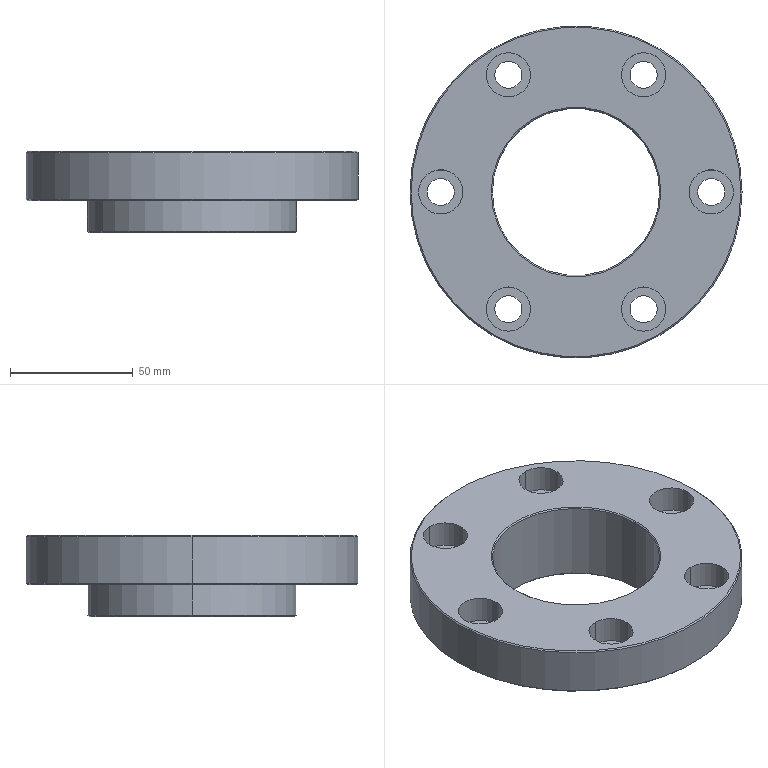Part | SolidWorks | features Chamfer 1, CirPattern 1, HoleWzd 1, Revolution 1 | 1 solid | 49 faces | box 135 x 135 x 33 mm | volume 218081 mm3 | cylinder 30 | cone 10 | plane 9 | commonest cylinder face diameters 11 x12 18 x12 68 x2 85 x2 135 x2
STEP:
#1=CARTESIAN_POINT('',(67.,0.,0.));
#2=VERTEX_POINT('',#1);
#3=CARTESIAN_POINT('',(-67.,0.,0.));
#4=VERTEX_POINT('',#3);
#5=CARTESIAN_POINT('',(0.,0.,0.));
#6=DIRECTION('',(0.,0.,1.));
#7=DIRECTION('',(1.,0.,0.));
#8=AXIS2_PLACEMENT_3D('',#5,#6,#7);
#9=CIRCLE('',#8,67.);
#10=EDGE_CURVE('',#2,#4,#9,.T.);
#11=ORIENTED_EDGE('',*,*,#10,.F.);
#12=CARTESIAN_POINT('',(67.5,0.,-0.5));
#13=VERTEX_POINT('',#12);
#14=CARTESIAN_POINT('',(67.5,0.,-0.5));
#15=DIRECTION('',(0.7071,0.,-0.7071));
#16=VECTOR('',#15,1000.);
#17=LINE('',#14,#16);
#18=EDGE_CURVE('',#2,#13,#17,.T.);
#19=ORIENTED_EDGE('',*,*,#18,.T.);
#20=CARTESIAN_POINT('',(-67.5,0.,-0.5));
#21=VERTEX_POINT('',#20);
#22=CARTESIAN_POINT('',(0.,0.,-0.5));
#23=DIRECTION('',(0.,0.,-1.));
#24=DIRECTION('',(1.,0.,0.));
#25=AXIS2_PLACEMENT_3D('',#22,#23,#24);
#26=CIRCLE('',#25,67.5);
#27=EDGE_CURVE('',#21,#13,#26,.T.);
#28=ORIENTED_EDGE('',*,*,#27,.F.);
#29=CARTESIAN_POINT('',(-67.5,0.,-0.5));
#30=DIRECTION('',(-0.7071,0.,-0.7071));
#31=VECTOR('',#30,1000.);
#32=LINE('',#29,#31);
#33=EDGE_CURVE('',#4,#21,#32,.T.);
#34=ORIENTED_EDGE('',*,*,#33,.F.);
#35=EDGE_LOOP('',(#11,#19,#28,#34));
#36=FACE_OUTER_BOUND('',#35,.T.);
#37=CARTESIAN_POINT('',(0.,0.,-0.5));
#38=DIRECTION('',(0.,0.,-1.));
#39=DIRECTION('',(-1.,0.,0.));
#40=AXIS2_PLACEMENT_3D('',#37,#38,#39);
#41=CONICAL_SURFACE('',#40,67.5,0.7854);
#42=ADVANCED_FACE('',(#36),#41,.T.);
#43=CARTESIAN_POINT('',(-34.,0.,-0.5));
#44=VERTEX_POINT('',#43);
#45=CARTESIAN_POINT('',(34.,0.,-0.5));
#46=VERTEX_POINT('',#45);
#47=CARTESIAN_POINT('',(0.,0.,-0.5));
#48=DIRECTION('',(0.,0.,1.));
#49=DIRECTION('',(1.,0.,0.));
#50=AXIS2_PLACEMENT_3D('',#47,#48,#49);
#51=CIRCLE('',#50,34.);
#52=EDGE_CURVE('',#44,#46,#51,.T.);
#53=ORIENTED_EDGE('',*,*,#52,.F.);
#54=CARTESIAN_POINT('',(-34.5,0.,0.));
#55=VERTEX_POINT('',#54);
#56=CARTESIAN_POINT('',(-34.5,0.,0.));
#57=DIRECTION('',(-0.7071,0.,0.7071));
#58=VECTOR('',#57,1000.);
#59=LINE('',#56,#58);
#60=EDGE_CURVE('',#44,#55,#59,.T.);
#61=ORIENTED_EDGE('',*,*,#60,.T.);
#62=CARTESIAN_POINT('',(34.5,0.,0.));
#63=VERTEX_POINT('',#62);
#64=CARTESIAN_POINT('',(0.,0.,0.));
#65=DIRECTION('',(0.,0.,-1.));
#66=DIRECTION('',(1.,0.,0.));
#67=AXIS2_PLACEMENT_3D('',#64,#65,#66);
#68=CIRCLE('',#67,34.5);
#69=EDGE_CURVE('',#63,#55,#68,.T.);
#70=ORIENTED_EDGE('',*,*,#69,.F.);
#71=CARTESIAN_POINT('',(34.5,0.,0.));
#72=DIRECTION('',(0.7071,0.,0.7071));
#73=VECTOR('',#72,1000.);
#74=LINE('',#71,#73);
#75=EDGE_CURVE('',#46,#63,#74,.T.);
#76=ORIENTED_EDGE('',*,*,#75,.F.);
#77=EDGE_LOOP('',(#53,#61,#70,#76));
#78=FACE_OUTER_BOUND('',#77,.T.);
#79=CARTESIAN_POINT('',(0.,0.,0.));
#80=DIRECTION('',(0.,0.,1.));
#81=DIRECTION('',(1.,0.,0.));
#82=AXIS2_PLACEMENT_3D('',#79,#80,#81);
#83=CONICAL_SURFACE('',#82,34.5,0.7854);
#84=ADVANCED_FACE('',(#78),#83,.F.);
#85=CARTESIAN_POINT('',(-67.,0.,-20.));
#86=VERTEX_POINT('',#85);
#87=CARTESIAN_POINT('',(67.,0.,-20.));
#88=VERTEX_POINT('',#87);
#89=CARTESIAN_POINT('',(0.,0.,-20.));
#90=DIRECTION('',(0.,0.,-1.));
#91=DIRECTION('',(-1.,0.,0.));
#92=AXIS2_PLACEMENT_3D('',#89,#90,#91);
#93=CIRCLE('',#92,67.);
#94=EDGE_CURVE('',#86,#88,#93,.T.);
#95=ORIENTED_EDGE('',*,*,#94,.F.);
#96=CARTESIAN_POINT('',(-67.5,0.,-19.5));
#97=VERTEX_POINT('',#96);
#98=CARTESIAN_POINT('',(-67.,0.,-20.));
#99=DIRECTION('',(-0.7071,0.,0.7071));
#100=VECTOR('',#99,1000.);
#101=LINE('',#98,#100);
#102=EDGE_CURVE('',#86,#97,#101,.T.);
#103=ORIENTED_EDGE('',*,*,#102,.T.);
#104=CARTESIAN_POINT('',(67.5,0.,-19.5));
#105=VERTEX_POINT('',#104);
#106=CARTESIAN_POINT('',(0.,0.,-19.5));
#107=DIRECTION('',(0.,0.,1.));
#108=DIRECTION('',(-1.,0.,0.));
#109=AXIS2_PLACEMENT_3D('',#106,#107,#108);
#110=CIRCLE('',#109,67.5);
#111=EDGE_CURVE('',#105,#97,#110,.T.);
#112=ORIENTED_EDGE('',*,*,#111,.F.);
#113=CARTESIAN_POINT('',(67.,0.,-20.));
#114=DIRECTION('',(0.7071,0.,0.7071));
#115=VECTOR('',#114,1000.);
#116=LINE('',#113,#115);
#117=EDGE_CURVE('',#88,#105,#116,.T.);
#118=ORIENTED_EDGE('',*,*,#117,.F.);
#119=EDGE_LOOP('',(#95,#103,#112,#118));
#120=FACE_OUTER_BOUND('',#119,.T.);
#121=CARTESIAN_POINT('',(0.,0.,-20.));
#122=DIRECTION('',(0.,0.,1.));
#123=DIRECTION('',(1.,0.,0.));
#124=AXIS2_PLACEMENT_3D('',#121,#122,#123);
#125=CONICAL_SURFACE('',#124,67.,0.7854);
#126=ADVANCED_FACE('',(#120),#125,.T.);
#127=CARTESIAN_POINT('',(-42.,0.,-33.));
#128=VERTEX_POINT('',#127);
#129=CARTESIAN_POINT('',(42.,0.,-33.));
#130=VERTEX_POINT('',#129);
#131=CARTESIAN_POINT('',(0.,0.,-33.));
#132=DIRECTION('',(0.,0.,-1.));
#133=DIRECTION('',(-1.,0.,0.));
#134=AXIS2_PLACEMENT_3D('',#131,#132,#133);
#135=CIRCLE('',#134,42.);
#136=EDGE_CURVE('',#128,#130,#135,.T.);
#137=ORIENTED_EDGE('',*,*,#136,.F.);
#138=CARTESIAN_POINT('',(-42.5,0.,-32.5));
#139=VERTEX_POINT('',#138);
#140=CARTESIAN_POINT('',(-42.,0.,-33.));
#141=DIRECTION('',(-0.7071,0.,0.7071));
#142=VECTOR('',#141,1000.);
#143=LINE('',#140,#142);
#144=EDGE_CURVE('',#128,#139,#143,.T.);
#145=ORIENTED_EDGE('',*,*,#144,.T.);
#146=CARTESIAN_POINT('',(42.5,0.,-32.5));
#147=VERTEX_POINT('',#146);
#148=CARTESIAN_POINT('',(0.,0.,-32.5));
#149=DIRECTION('',(0.,0.,1.));
#150=DIRECTION('',(-1.,0.,0.));
#151=AXIS2_PLACEMENT_3D('',#148,#149,#150);
#152=CIRCLE('',#151,42.5);
#153=EDGE_CURVE('',#147,#139,#152,.T.);
#154=ORIENTED_EDGE('',*,*,#153,.F.);
#155=CARTESIAN_POINT('',(42.,0.,-33.));
#156=DIRECTION('',(0.7071,0.,0.7071));
#157=VECTOR('',#156,1000.);
#158=LINE('',#155,#157);
#159=EDGE_CURVE('',#130,#147,#158,.T.);
#160=ORIENTED_EDGE('',*,*,#159,.F.);
#161=EDGE_LOOP('',(#137,#145,#154,#160));
#162=FACE_OUTER_BOUND('',#161,.T.);
#163=CARTESIAN_POINT('',(0.,0.,-33.));
#164=DIRECTION('',(0.,0.,1.));
#165=DIRECTION('',(1.,0.,0.));
#166=AXIS2_PLACEMENT_3D('',#163,#164,#165);
#167=CONICAL_SURFACE('',#166,42.,0.7854);
#168=ADVANCED_FACE('',(#162),#167,.T.);
#169=CARTESIAN_POINT('',(34.,0.,-32.5));
#170=VERTEX_POINT('',#169);
#171=CARTESIAN_POINT('',(-34.,0.,-32.5));
#172=VERTEX_POINT('',#171);
#173=CARTESIAN_POINT('',(0.,0.,-32.5));
#174=DIRECTION('',(0.,0.,-1.));
#175=DIRECTION('',(-1.,0.,0.));
#176=AXIS2_PLACEMENT_3D('',#173,#174,#175);
#177=CIRCLE('',#176,34.);
#178=EDGE_CURVE('',#170,#172,#177,.T.);
#179=ORIENTED_EDGE('',*,*,#178,.F.);
#180=CARTESIAN_POINT('',(34.5,0.,-33.));
#181=VERTEX_POINT('',#180);
#182=CARTESIAN_POINT('',(34.,0.,-32.5));
#183=DIRECTION('',(0.7071,0.,-0.7071));
#184=VECTOR('',#183,1000.);
#185=LINE('',#182,#184);
#186=EDGE_CURVE('',#170,#181,#185,.T.);
#187=ORIENTED_EDGE('',*,*,#186,.T.);
#188=CARTESIAN_POINT('',(-34.5,0.,-33.));
#189=VERTEX_POINT('',#188);
#190=CARTESIAN_POINT('',(0.,0.,-33.));
#191=DIRECTION('',(0.,0.,1.));
#192=DIRECTION('',(-1.,0.,0.));
#193=AXIS2_PLACEMENT_3D('',#190,#191,#192);
#194=CIRCLE('',#193,34.5);
#195=EDGE_CURVE('',#189,#181,#194,.T.);
#196=ORIENTED_EDGE('',*,*,#195,.F.);
#197=CARTESIAN_POINT('',(-34.,0.,-32.5));
#198=DIRECTION('',(-0.7071,0.,-0.7071));
#199=VECTOR('',#198,1000.);
#200=LINE('',#197,#199);
#201=EDGE_CURVE('',#172,#189,#200,.T.);
#202=ORIENTED_EDGE('',*,*,#201,.F.);
#203=EDGE_LOOP('',(#179,#187,#196,#202));
#204=FACE_OUTER_BOUND('',#203,.T.);
#205=CARTESIAN_POINT('',(0.,0.,-32.5));
#206=DIRECTION('',(0.,0.,-1.));
#207=DIRECTION('',(-1.,0.,0.));
#208=AXIS2_PLACEMENT_3D('',#205,#206,#207);
#209=CONICAL_SURFACE('',#208,34.,0.7854);
#210=ADVANCED_FACE('',(#204),#209,.F.);
#211=CARTESIAN_POINT('',(27.5,56.631,-11.));
#212=VERTEX_POINT('',#211);
#213=CARTESIAN_POINT('',(27.5,38.631,-11.));
#214=VERTEX_POINT('',#213);
#215=CARTESIAN_POINT('',(27.5,47.631,-11.));
#216=DIRECTION('',(0.,0.,1.));
#217=DIRECTION('',(0.,-1.,0.));
#218=AXIS2_PLACEMENT_3D('',#215,#216,#217);
#219=CIRCLE('',#218,9.);
#220=EDGE_CURVE('',#212,#214,#219,.T.);
#221=ORIENTED_EDGE('',*,*,#220,.F.);
#222=CARTESIAN_POINT('',(27.5,56.631,0.));
#223=VERTEX_POINT('',#222);
#224=CARTESIAN_POINT('',(27.5,56.631,0.));
#225=DIRECTION('',(0.,0.,1.));
#226=VECTOR('',#225,1000.);
#227=LINE('',#224,#226);
#228=EDGE_CURVE('',#212,#223,#227,.T.);
#229=ORIENTED_EDGE('',*,*,#228,.T.);
#230=CARTESIAN_POINT('',(27.5,38.631,0.));
#231=VERTEX_POINT('',#230);
#232=CARTESIAN_POINT('',(27.5,47.631,0.));
#233=DIRECTION('',(0.,0.,1.));
#234=DIRECTION('',(0.,-1.,0.));
#235=AXIS2_PLACEMENT_3D('',#232,#233,#234);
#236=CIRCLE('',#235,9.);
#237=EDGE_CURVE('',#223,#231,#236,.T.);
#238=ORIENTED_EDGE('',*,*,#237,.T.);
#239=CARTESIAN_POINT('',(27.5,38.631,0.));
#240=DIRECTION('',(0.,0.,1.));
#241=VECTOR('',#240,1000.);
#242=LINE('',#239,#241);
#243=EDGE_CURVE('',#214,#231,#242,.T.);
#244=ORIENTED_EDGE('',*,*,#243,.F.);
#245=EDGE_LOOP('',(#221,#229,#238,#244));
#246=FACE_OUTER_BOUND('',#245,.T.);
#247=CARTESIAN_POINT('',(27.5,47.631,0.));
#248=DIRECTION('',(0.,0.,1.));
#249=DIRECTION('',(0.,-1.,0.));
#250=AXIS2_PLACEMENT_3D('',#247,#248,#249);
#251=CYLINDRICAL_SURFACE('',#250,9.);
#252=ADVANCED_FACE('',(#246),#251,.F.);
#253=CARTESIAN_POINT('',(27.5,42.131,-20.));
#254=VERTEX_POINT('',#253);
#255=CARTESIAN_POINT('',(27.5,53.131,-20.));
#256=VERTEX_POINT('',#255);
#257=CARTESIAN_POINT('',(27.5,47.631,-20.));
#258=DIRECTION('',(0.,0.,-1.));
#259=DIRECTION('',(-1.,0.,0.));
#260=AXIS2_PLACEMENT_3D('',#257,#258,#259);
#261=CIRCLE('',#260,5.5);
#262=EDGE_CURVE('',#254,#256,#261,.T.);
#263=ORIENTED_EDGE('',*,*,#262,.T.);
#264=CARTESIAN_POINT('',(27.5,53.131,-11.));
#265=VERTEX_POINT('',#264);
#266=CARTESIAN_POINT('',(27.5,53.131,0.));
#267=DIRECTION('',(0.,0.,1.));
#268=VECTOR('',#267,1000.);
#269=LINE('',#266,#268);
#270=EDGE_CURVE('',#256,#265,#269,.T.);
#271=ORIENTED_EDGE('',*,*,#270,.T.);
#272=CARTESIAN_POINT('',(27.5,42.131,-11.));
#273=VERTEX_POINT('',#272);
#274=CARTESIAN_POINT('',(27.5,47.631,-11.));
#275=DIRECTION('',(0.,0.,1.));
#276=DIRECTION('',(0.,-1.,0.));
#277=AXIS2_PLACEMENT_3D('',#274,#275,#276);
#278=CIRCLE('',#277,5.5);
#279=EDGE_CURVE('',#265,#273,#278,.T.);
#280=ORIENTED_EDGE('',*,*,#279,.T.);
#281=CARTESIAN_POINT('',(27.5,42.131,0.));
#282=DIRECTION('',(0.,0.,1.));
#283=VECTOR('',#282,1000.);
#284=LINE('',#281,#283);
#285=EDGE_CURVE('',#254,#273,#284,.T.);
#286=ORIENTED_EDGE('',*,*,#285,.F.);
#287=EDGE_LOOP('',(#263,#271,#280,#286));
#288=FACE_OUTER_BOUND('',#287,.T.);
#289=CARTESIAN_POINT('',(27.5,47.631,0.));
#290=DIRECTION('',(0.,0.,1.));
#291=DIRECTION('',(0.,-1.,0.));
#292=AXIS2_PLACEMENT_3D('',#289,#290,#291);
#293=CYLINDRICAL_SURFACE('',#292,5.5);
#294=ADVANCED_FACE('',(#288),#293,.F.);
#295=CARTESIAN_POINT('',(-27.5,56.631,-11.));
#296=VERTEX_POINT('',#295);
#297=CARTESIAN_POINT('',(-27.5,38.631,-11.));
#298=VERTEX_POINT('',#297);
#299=CARTESIAN_POINT('',(-27.5,47.631,-11.));
#300=DIRECTION('',(0.,0.,1.));
#301=DIRECTION('',(0.,-1.,0.));
#302=AXIS2_PLACEMENT_3D('',#299,#300,#301);
#303=CIRCLE('',#302,9.);
#304=EDGE_CURVE('',#296,#298,#303,.T.);
#305=ORIENTED_EDGE('',*,*,#304,.F.);
#306=CARTESIAN_POINT('',(-27.5,56.631,0.));
#307=VERTEX_POINT('',#306);
#308=CARTESIAN_POINT('',(-27.5,56.631,0.));
#309=DIRECTION('',(0.,0.,1.));
#310=VECTOR('',#309,1000.);
#311=LINE('',#308,#310);
#312=EDGE_CURVE('',#296,#307,#311,.T.);
#313=ORIENTED_EDGE('',*,*,#312,.T.);
#314=CARTESIAN_POINT('',(-27.5,38.631,0.));
#315=VERTEX_POINT('',#314);
#316=CARTESIAN_POINT('',(-27.5,47.631,0.));
#317=DIRECTION('',(0.,0.,1.));
#318=DIRECTION('',(0.,-1.,0.));
#319=AXIS2_PLACEMENT_3D('',#316,#317,#318);
#320=CIRCLE('',#319,9.);
#321=EDGE_CURVE('',#307,#315,#320,.T.);
#322=ORIENTED_EDGE('',*,*,#321,.T.);
#323=CARTESIAN_POINT('',(-27.5,38.631,0.));
#324=DIRECTION('',(0.,0.,1.));
#325=VECTOR('',#324,1000.);
#326=LINE('',#323,#325);
#327=EDGE_CURVE('',#298,#315,#326,.T.);
#328=ORIENTED_EDGE('',*,*,#327,.F.);
#329=EDGE_LOOP('',(#305,#313,#322,#328));
#330=FACE_OUTER_BOUND('',#329,.T.);
#331=CARTESIAN_POINT('',(-27.5,47.631,0.));
#332=DIRECTION('',(0.,0.,1.));
#333=DIRECTION('',(0.,-1.,0.));
#334=AXIS2_PLACEMENT_3D('',#331,#332,#333);
#335=CYLINDRICAL_SURFACE('',#334,9.);
#336=ADVANCED_FACE('',(#330),#335,.F.);
#337=CARTESIAN_POINT('',(-27.5,42.131,-20.));
#338=VERTEX_POINT('',#337);
#339=CARTESIAN_POINT('',(-27.5,53.131,-20.));
#340=VERTEX_POINT('',#339);
#341=CARTESIAN_POINT('',(-27.5,47.631,-20.));
#342=DIRECTION('',(0.,0.,-1.));
#343=DIRECTION('',(-1.,0.,0.));
#344=AXIS2_PLACEMENT_3D('',#341,#342,#343);
#345=CIRCLE('',#344,5.5);
#346=EDGE_CURVE('',#338,#340,#345,.T.);
#347=ORIENTED_EDGE('',*,*,#346,.T.);
#348=CARTESIAN_POINT('',(-27.5,53.131,-11.));
#349=VERTEX_POINT('',#348);
#350=CARTESIAN_POINT('',(-27.5,53.131,0.));
#351=DIRECTION('',(0.,0.,1.));
#352=VECTOR('',#351,1000.);
#353=LINE('',#350,#352);
#354=EDGE_CURVE('',#340,#349,#353,.T.);
#355=ORIENTED_EDGE('',*,*,#354,.T.);
#356=CARTESIAN_POINT('',(-27.5,42.131,-11.));
#357=VERTEX_POINT('',#356);
#358=CARTESIAN_POINT('',(-27.5,47.631,-11.));
#359=DIRECTION('',(0.,0.,1.));
#360=DIRECTION('',(0.,-1.,0.));
#361=AXIS2_PLACEMENT_3D('',#358,#359,#360);
#362=CIRCLE('',#361,5.5);
#363=EDGE_CURVE('',#349,#357,#362,.T.);
#364=ORIENTED_EDGE('',*,*,#363,.T.);
#365=CARTESIAN_POINT('',(-27.5,42.131,0.));
#366=DIRECTION('',(0.,0.,1.));
#367=VECTOR('',#366,1000.);
#368=LINE('',#365,#367);
#369=EDGE_CURVE('',#338,#357,#368,.T.);
#370=ORIENTED_EDGE('',*,*,#369,.F.);
#371=EDGE_LOOP('',(#347,#355,#364,#370));
#372=FACE_OUTER_BOUND('',#371,.T.);
#373=CARTESIAN_POINT('',(-27.5,47.631,0.));
#374=DIRECTION('',(0.,0.,1.));
#375=DIRECTION('',(0.,-1.,0.));
#376=AXIS2_PLACEMENT_3D('',#373,#374,#375);
#377=CYLINDRICAL_SURFACE('',#376,5.5);
#378=ADVANCED_FACE('',(#372),#377,.F.);
#379=CARTESIAN_POINT('',(-64.,0.,-11.));
#380=VERTEX_POINT('',#379);
#381=CARTESIAN_POINT('',(-46.,0.,-11.));
#382=VERTEX_POINT('',#381);
#383=CARTESIAN_POINT('',(-55.,0.,-11.));
#384=DIRECTION('',(0.,0.,1.));
#385=DIRECTION('',(1.,0.,0.));
#386=AXIS2_PLACEMENT_3D('',#383,#384,#385);
#387=CIRCLE('',#386,9.);
#388=EDGE_CURVE('',#380,#382,#387,.T.);
#389=ORIENTED_EDGE('',*,*,#388,.F.);
#390=CARTESIAN_POINT('',(-64.,0.,0.));
#391=VERTEX_POINT('',#390);
#392=CARTESIAN_POINT('',(-64.,0.,0.));
#393=DIRECTION('',(0.,0.,1.));
#394=VECTOR('',#393,1000.);
#395=LINE('',#392,#394);
#396=EDGE_CURVE('',#380,#391,#395,.T.);
#397=ORIENTED_EDGE('',*,*,#396,.T.);
#398=CARTESIAN_POINT('',(-46.,0.,0.));
#399=VERTEX_POINT('',#398);
#400=CARTESIAN_POINT('',(-55.,0.,0.));
#401=DIRECTION('',(0.,0.,1.));
#402=DIRECTION('',(1.,0.,0.));
#403=AXIS2_PLACEMENT_3D('',#400,#401,#402);
#404=CIRCLE('',#403,9.);
#405=EDGE_CURVE('',#391,#399,#404,.T.);
#406=ORIENTED_EDGE('',*,*,#405,.T.);
#407=CARTESIAN_POINT('',(-46.,0.,0.));
#408=DIRECTION('',(0.,0.,1.));
#409=VECTOR('',#408,1000.);
#410=LINE('',#407,#409);
#411=EDGE_CURVE('',#382,#399,#410,.T.);
#412=ORIENTED_EDGE('',*,*,#411,.F.);
#413=EDGE_LOOP('',(#389,#397,#406,#412));
#414=FACE_OUTER_BOUND('',#413,.T.);
#415=CARTESIAN_POINT('',(-55.,0.,0.));
#416=DIRECTION('',(0.,0.,1.));
#417=DIRECTION('',(1.,0.,0.));
#418=AXIS2_PLACEMENT_3D('',#415,#416,#417);
#419=CYLINDRICAL_SURFACE('',#418,9.);
#420=ADVANCED_FACE('',(#414),#419,.F.);
#421=CARTESIAN_POINT('',(-49.5,0.,-20.));
#422=VERTEX_POINT('',#421);
#423=CARTESIAN_POINT('',(-60.5,0.,-20.));
#424=VERTEX_POINT('',#423);
#425=CARTESIAN_POINT('',(-55.,0.,-20.));
#426=DIRECTION('',(0.,0.,-1.));
#427=DIRECTION('',(-1.,0.,0.));
#428=AXIS2_PLACEMENT_3D('',#425,#426,#427);
#429=CIRCLE('',#428,5.5);
#430=EDGE_CURVE('',#422,#424,#429,.T.);
#431=ORIENTED_EDGE('',*,*,#430,.T.);
#432=CARTESIAN_POINT('',(-60.5,0.,-11.));
#433=VERTEX_POINT('',#432);
#434=CARTESIAN_POINT('',(-60.5,0.,0.));
#435=DIRECTION('',(0.,0.,1.));
#436=VECTOR('',#435,1000.);
#437=LINE('',#434,#436);
#438=EDGE_CURVE('',#424,#433,#437,.T.);
#439=ORIENTED_EDGE('',*,*,#438,.T.);
#440=CARTESIAN_POINT('',(-49.5,0.,-11.));
#441=VERTEX_POINT('',#440);
#442=CARTESIAN_POINT('',(-55.,0.,-11.));
#443=DIRECTION('',(0.,0.,1.));
#444=DIRECTION('',(1.,0.,0.));
#445=AXIS2_PLACEMENT_3D('',#442,#443,#444);
#446=CIRCLE('',#445,5.5);
#447=EDGE_CURVE('',#433,#441,#446,.T.);
#448=ORIENTED_EDGE('',*,*,#447,.T.);
#449=CARTESIAN_POINT('',(-49.5,0.,0.));
#450=DIRECTION('',(0.,0.,1.));
#451=VECTOR('',#450,1000.);
#452=LINE('',#449,#451);
#453=EDGE_CURVE('',#422,#441,#452,.T.);
#454=ORIENTED_EDGE('',*,*,#453,.F.);
#455=EDGE_LOOP('',(#431,#439,#448,#454));
#456=FACE_OUTER_BOUND('',#455,.T.);
#457=CARTESIAN_POINT('',(-55.,0.,0.));
#458=DIRECTION('',(0.,0.,1.));
#459=DIRECTION('',(1.,0.,0.));
#460=AXIS2_PLACEMENT_3D('',#457,#458,#459);
#461=CYLINDRICAL_SURFACE('',#460,5.5);
#462=ADVANCED_FACE('',(#456),#461,.F.);
#463=CARTESIAN_POINT('',(-27.5,-38.631,-11.));
#464=VERTEX_POINT('',#463);
#465=CARTESIAN_POINT('',(-27.5,-56.631,-11.));
#466=VERTEX_POINT('',#465);
#467=CARTESIAN_POINT('',(-27.5,-47.631,-11.));
#468=DIRECTION('',(0.,0.,1.));
#469=DIRECTION('',(0.,-1.,0.));
#470=AXIS2_PLACEMENT_3D('',#467,#468,#469);
#471=CIRCLE('',#470,9.);
#472=EDGE_CURVE('',#464,#466,#471,.T.);
#473=ORIENTED_EDGE('',*,*,#472,.F.);
#474=CARTESIAN_POINT('',(-27.5,-38.631,0.));
#475=VERTEX_POINT('',#474);
#476=CARTESIAN_POINT('',(-27.5,-38.631,0.));
#477=DIRECTION('',(0.,0.,1.));
#478=VECTOR('',#477,1000.);
#479=LINE('',#476,#478);
#480=EDGE_CURVE('',#464,#475,#479,.T.);
#481=ORIENTED_EDGE('',*,*,#480,.T.);
#482=CARTESIAN_POINT('',(-27.5,-56.631,0.));
#483=VERTEX_POINT('',#482);
#484=CARTESIAN_POINT('',(-27.5,-47.631,0.));
#485=DIRECTION('',(0.,0.,1.));
#486=DIRECTION('',(0.,-1.,0.));
#487=AXIS2_PLACEMENT_3D('',#484,#485,#486);
#488=CIRCLE('',#487,9.);
#489=EDGE_CURVE('',#475,#483,#488,.T.);
#490=ORIENTED_EDGE('',*,*,#489,.T.);
#491=CARTESIAN_POINT('',(-27.5,-56.631,0.));
#492=DIRECTION('',(0.,0.,1.));
#493=VECTOR('',#492,1000.);
#494=LINE('',#491,#493);
#495=EDGE_CURVE('',#466,#483,#494,.T.);
#496=ORIENTED_EDGE('',*,*,#495,.F.);
#497=EDGE_LOOP('',(#473,#481,#490,#496));
#498=FACE_OUTER_BOUND('',#497,.T.);
#499=CARTESIAN_POINT('',(-27.5,-47.631,0.));
#500=DIRECTION('',(0.,0.,1.));
#501=DIRECTION('',(0.,-1.,0.));
#502=AXIS2_PLACEMENT_3D('',#499,#500,#501);
#503=CYLINDRICAL_SURFACE('',#502,9.);
#504=ADVANCED_FACE('',(#498),#503,.F.);
#505=CARTESIAN_POINT('',(-27.5,-53.131,-20.));
#506=VERTEX_POINT('',#505);
#507=CARTESIAN_POINT('',(-27.5,-42.131,-20.));
#508=VERTEX_POINT('',#507);
#509=CARTESIAN_POINT('',(-27.5,-47.631,-20.));
#510=DIRECTION('',(0.,0.,-1.));
#511=DIRECTION('',(-1.,0.,0.));
#512=AXIS2_PLACEMENT_3D('',#509,#510,#511);
#513=CIRCLE('',#512,5.5);
#514=EDGE_CURVE('',#506,#508,#513,.T.);
#515=ORIENTED_EDGE('',*,*,#514,.T.);
#516=CARTESIAN_POINT('',(-27.5,-42.131,-11.));
#517=VERTEX_POINT('',#516);
#518=CARTESIAN_POINT('',(-27.5,-42.131,0.));
#519=DIRECTION('',(0.,0.,1.));
#520=VECTOR('',#519,1000.);
#521=LINE('',#518,#520);
#522=EDGE_CURVE('',#508,#517,#521,.T.);
#523=ORIENTED_EDGE('',*,*,#522,.T.);
#524=CARTESIAN_POINT('',(-27.5,-53.131,-11.));
#525=VERTEX_POINT('',#524);
#526=CARTESIAN_POINT('',(-27.5,-47.631,-11.));
#527=DIRECTION('',(0.,0.,1.));
#528=DIRECTION('',(0.,-1.,0.));
#529=AXIS2_PLACEMENT_3D('',#526,#527,#528);
#530=CIRCLE('',#529,5.5);
#531=EDGE_CURVE('',#517,#525,#530,.T.);
#532=ORIENTED_EDGE('',*,*,#531,.T.);
#533=CARTESIAN_POINT('',(-27.5,-53.131,0.));
#534=DIRECTION('',(0.,0.,1.));
#535=VECTOR('',#534,1000.);
#536=LINE('',#533,#535);
#537=EDGE_CURVE('',#506,#525,#536,.T.);
#538=ORIENTED_EDGE('',*,*,#537,.F.);
#539=EDGE_LOOP('',(#515,#523,#532,#538));
#540=FACE_OUTER_BOUND('',#539,.T.);
#541=CARTESIAN_POINT('',(-27.5,-47.631,0.));
#542=DIRECTION('',(0.,0.,1.));
#543=DIRECTION('',(0.,-1.,0.));
#544=AXIS2_PLACEMENT_3D('',#541,#542,#543);
#545=CYLINDRICAL_SURFACE('',#544,5.5);
#546=ADVANCED_FACE('',(#540),#545,.F.);
#547=CARTESIAN_POINT('',(27.5,-38.631,-11.));
#548=VERTEX_POINT('',#547);
#549=CARTESIAN_POINT('',(27.5,-56.631,-11.));
#550=VERTEX_POINT('',#549);
#551=CARTESIAN_POINT('',(27.5,-47.631,-11.));
#552=DIRECTION('',(0.,0.,1.));
#553=DIRECTION('',(0.,-1.,0.));
#554=AXIS2_PLACEMENT_3D('',#551,#552,#553);
#555=CIRCLE('',#554,9.);
#556=EDGE_CURVE('',#548,#550,#555,.T.);
#557=ORIENTED_EDGE('',*,*,#556,.F.);
#558=CARTESIAN_POINT('',(27.5,-38.631,0.));
#559=VERTEX_POINT('',#558);
#560=CARTESIAN_POINT('',(27.5,-38.631,0.));
#561=DIRECTION('',(0.,0.,1.));
#562=VECTOR('',#561,1000.);
#563=LINE('',#560,#562);
#564=EDGE_CURVE('',#548,#559,#563,.T.);
#565=ORIENTED_EDGE('',*,*,#564,.T.);
#566=CARTESIAN_POINT('',(27.5,-56.631,0.));
#567=VERTEX_POINT('',#566);
#568=CARTESIAN_POINT('',(27.5,-47.631,0.));
#569=DIRECTION('',(0.,0.,1.));
#570=DIRECTION('',(0.,-1.,0.));
#571=AXIS2_PLACEMENT_3D('',#568,#569,#570);
#572=CIRCLE('',#571,9.);
#573=EDGE_CURVE('',#559,#567,#572,.T.);
#574=ORIENTED_EDGE('',*,*,#573,.T.);
#575=CARTESIAN_POINT('',(27.5,-56.631,0.));
#576=DIRECTION('',(0.,0.,1.));
#577=VECTOR('',#576,1000.);
#578=LINE('',#575,#577);
#579=EDGE_CURVE('',#550,#567,#578,.T.);
#580=ORIENTED_EDGE('',*,*,#579,.F.);
#581=EDGE_LOOP('',(#557,#565,#574,#580));
#582=FACE_OUTER_BOUND('',#581,.T.);
#583=CARTESIAN_POINT('',(27.5,-47.631,0.));
#584=DIRECTION('',(0.,0.,1.));
#585=DIRECTION('',(0.,-1.,0.));
#586=AXIS2_PLACEMENT_3D('',#583,#584,#585);
#587=CYLINDRICAL_SURFACE('',#586,9.);
#588=ADVANCED_FACE('',(#582),#587,.F.);
#589=CARTESIAN_POINT('',(27.5,-53.131,-20.));
#590=VERTEX_POINT('',#589);
#591=CARTESIAN_POINT('',(27.5,-42.131,-20.));
#592=VERTEX_POINT('',#591);
#593=CARTESIAN_POINT('',(27.5,-47.631,-20.));
#594=DIRECTION('',(0.,0.,-1.));
#595=DIRECTION('',(-1.,0.,0.));
#596=AXIS2_PLACEMENT_3D('',#593,#594,#595);
#597=CIRCLE('',#596,5.5);
#598=EDGE_CURVE('',#590,#592,#597,.T.);
#599=ORIENTED_EDGE('',*,*,#598,.T.);
#600=CARTESIAN_POINT('',(27.5,-42.131,-11.));
#601=VERTEX_POINT('',#600);
#602=CARTESIAN_POINT('',(27.5,-42.131,0.));
#603=DIRECTION('',(0.,0.,1.));
#604=VECTOR('',#603,1000.);
#605=LINE('',#602,#604);
#606=EDGE_CURVE('',#592,#601,#605,.T.);
#607=ORIENTED_EDGE('',*,*,#606,.T.);
#608=CARTESIAN_POINT('',(27.5,-53.131,-11.));
#609=VERTEX_POINT('',#608);
#610=CARTESIAN_POINT('',(27.5,-47.631,-11.));
#611=DIRECTION('',(0.,0.,1.));
#612=DIRECTION('',(0.,-1.,0.));
#613=AXIS2_PLACEMENT_3D('',#610,#611,#612);
#614=CIRCLE('',#613,5.5);
#615=EDGE_CURVE('',#601,#609,#614,.T.);
#616=ORIENTED_EDGE('',*,*,#615,.T.);
#617=CARTESIAN_POINT('',(27.5,-53.131,0.));
#618=DIRECTION('',(0.,0.,1.));
#619=VECTOR('',#618,1000.);
#620=LINE('',#617,#619);
#621=EDGE_CURVE('',#590,#609,#620,.T.);
#622=ORIENTED_EDGE('',*,*,#621,.F.);
#623=EDGE_LOOP('',(#599,#607,#616,#622));
#624=FACE_OUTER_BOUND('',#623,.T.);
#625=CARTESIAN_POINT('',(27.5,-47.631,0.));
#626=DIRECTION('',(0.,0.,1.));
#627=DIRECTION('',(0.,-1.,0.));
#628=AXIS2_PLACEMENT_3D('',#625,#626,#627);
#629=CYLINDRICAL_SURFACE('',#628,5.5);
#630=ADVANCED_FACE('',(#624),#629,.F.);
#631=CARTESIAN_POINT('',(46.,0.,-11.));
#632=VERTEX_POINT('',#631);
#633=CARTESIAN_POINT('',(64.,0.,-11.));
#634=VERTEX_POINT('',#633);
#635=CARTESIAN_POINT('',(55.,0.,-11.));
#636=DIRECTION('',(0.,0.,1.));
#637=DIRECTION('',(1.,0.,0.));
#638=AXIS2_PLACEMENT_3D('',#635,#636,#637);
#639=CIRCLE('',#638,9.);
#640=EDGE_CURVE('',#632,#634,#639,.T.);
#641=ORIENTED_EDGE('',*,*,#640,.F.);
#642=CARTESIAN_POINT('',(46.,0.,0.));
#643=VERTEX_POINT('',#642);
#644=CARTESIAN_POINT('',(46.,0.,0.));
#645=DIRECTION('',(0.,0.,1.));
#646=VECTOR('',#645,1000.);
#647=LINE('',#644,#646);
#648=EDGE_CURVE('',#632,#643,#647,.T.);
#649=ORIENTED_EDGE('',*,*,#648,.T.);
#650=CARTESIAN_POINT('',(64.,0.,0.));
#651=VERTEX_POINT('',#650);
#652=CARTESIAN_POINT('',(55.,0.,0.));
#653=DIRECTION('',(0.,0.,1.));
#654=DIRECTION('',(1.,0.,0.));
#655=AXIS2_PLACEMENT_3D('',#652,#653,#654);
#656=CIRCLE('',#655,9.);
#657=EDGE_CURVE('',#643,#651,#656,.T.);
#658=ORIENTED_EDGE('',*,*,#657,.T.);
#659=CARTESIAN_POINT('',(64.,0.,0.));
#660=DIRECTION('',(0.,0.,1.));
#661=VECTOR('',#660,1000.);
#662=LINE('',#659,#661);
#663=EDGE_CURVE('',#634,#651,#662,.T.);
#664=ORIENTED_EDGE('',*,*,#663,.F.);
#665=EDGE_LOOP('',(#641,#649,#658,#664));
#666=FACE_OUTER_BOUND('',#665,.T.);
#667=CARTESIAN_POINT('',(55.,0.,0.));
#668=DIRECTION('',(0.,0.,1.));
#669=DIRECTION('',(1.,0.,0.));
#670=AXIS2_PLACEMENT_3D('',#667,#668,#669);
#671=CYLINDRICAL_SURFACE('',#670,9.);
#672=ADVANCED_FACE('',(#666),#671,.F.);
#673=CARTESIAN_POINT('',(60.5,0.,-20.));
#674=VERTEX_POINT('',#673);
#675=CARTESIAN_POINT('',(49.5,0.,-20.));
#676=VERTEX_POINT('',#675);
#677=CARTESIAN_POINT('',(55.,0.,-20.));
#678=DIRECTION('',(0.,0.,-1.));
#679=DIRECTION('',(-1.,0.,0.));
#680=AXIS2_PLACEMENT_3D('',#677,#678,#679);
#681=CIRCLE('',#680,5.5);
#682=EDGE_CURVE('',#674,#676,#681,.T.);
#683=ORIENTED_EDGE('',*,*,#682,.T.);
#684=CARTESIAN_POINT('',(49.5,0.,-11.));
#685=VERTEX_POINT('',#684);
#686=CARTESIAN_POINT('',(49.5,0.,0.));
#687=DIRECTION('',(0.,0.,1.));
#688=VECTOR('',#687,1000.);
#689=LINE('',#686,#688);
#690=EDGE_CURVE('',#676,#685,#689,.T.);
#691=ORIENTED_EDGE('',*,*,#690,.T.);
#692=CARTESIAN_POINT('',(60.5,0.,-11.));
#693=VERTEX_POINT('',#692);
#694=CARTESIAN_POINT('',(55.,0.,-11.));
#695=DIRECTION('',(0.,0.,1.));
#696=DIRECTION('',(1.,0.,0.));
#697=AXIS2_PLACEMENT_3D('',#694,#695,#696);
#698=CIRCLE('',#697,5.5);
#699=EDGE_CURVE('',#685,#693,#698,.T.);
#700=ORIENTED_EDGE('',*,*,#699,.T.);
#701=CARTESIAN_POINT('',(60.5,0.,0.));
#702=DIRECTION('',(0.,0.,1.));
#703=VECTOR('',#702,1000.);
#704=LINE('',#701,#703);
#705=EDGE_CURVE('',#674,#693,#704,.T.);
#706=ORIENTED_EDGE('',*,*,#705,.F.);
#707=EDGE_LOOP('',(#683,#691,#700,#706));
#708=FACE_OUTER_BOUND('',#707,.T.);
#709=CARTESIAN_POINT('',(55.,0.,0.));
#710=DIRECTION('',(0.,0.,1.));
#711=DIRECTION('',(1.,0.,0.));
#712=AXIS2_PLACEMENT_3D('',#709,#710,#711);
#713=CYLINDRICAL_SURFACE('',#712,5.5);
#714=ADVANCED_FACE('',(#708),#713,.F.);
#715=ORIENTED_EDGE('',*,*,#52,.T.);
#716=CARTESIAN_POINT('',(34.,0.,0.));
#717=DIRECTION('',(0.,0.,-1.));
#718=VECTOR('',#717,1000.);
#719=LINE('',#716,#718);
#720=EDGE_CURVE('',#46,#170,#719,.T.);
#721=ORIENTED_EDGE('',*,*,#720,.T.);
#722=ORIENTED_EDGE('',*,*,#178,.T.);
#723=CARTESIAN_POINT('',(-34.,0.,0.));
#724=DIRECTION('',(0.,0.,-1.));
#725=VECTOR('',#724,1000.);
#726=LINE('',#723,#725);
#727=EDGE_CURVE('',#44,#172,#726,.T.);
#728=ORIENTED_EDGE('',*,*,#727,.F.);
#729=EDGE_LOOP('',(#715,#721,#722,#728));
#730=FACE_OUTER_BOUND('',#729,.T.);
#731=CARTESIAN_POINT('',(0.,0.,0.));
#732=DIRECTION('',(0.,0.,-1.));
#733=DIRECTION('',(-1.,0.,0.));
#734=AXIS2_PLACEMENT_3D('',#731,#732,#733);
#735=CYLINDRICAL_SURFACE('',#734,34.);
#736=ADVANCED_FACE('',(#730),#735,.F.);
#737=CARTESIAN_POINT('',(-42.5,0.,-20.));
#738=VERTEX_POINT('',#737);
#739=CARTESIAN_POINT('',(42.5,0.,-20.));
#740=VERTEX_POINT('',#739);
#741=CARTESIAN_POINT('',(0.,0.,-20.));
#742=DIRECTION('',(0.,0.,-1.));
#743=DIRECTION('',(-1.,0.,0.));
#744=AXIS2_PLACEMENT_3D('',#741,#742,#743);
#745=CIRCLE('',#744,42.5);
#746=EDGE_CURVE('',#738,#740,#745,.T.);
#747=ORIENTED_EDGE('',*,*,#746,.T.);
#748=CARTESIAN_POINT('',(42.5,0.,0.));
#749=DIRECTION('',(0.,0.,-1.));
#750=VECTOR('',#749,1000.);
#751=LINE('',#748,#750);
#752=EDGE_CURVE('',#740,#147,#751,.T.);
#753=ORIENTED_EDGE('',*,*,#752,.T.);
#754=ORIENTED_EDGE('',*,*,#153,.T.);
#755=CARTESIAN_POINT('',(-42.5,0.,0.));
#756=DIRECTION('',(0.,0.,-1.));
#757=VECTOR('',#756,1000.);
#758=LINE('',#755,#757);
#759=EDGE_CURVE('',#738,#139,#758,.T.);
#760=ORIENTED_EDGE('',*,*,#759,.F.);
#761=EDGE_LOOP('',(#747,#753,#754,#760));
#762=FACE_OUTER_BOUND('',#761,.T.);
#763=CARTESIAN_POINT('',(0.,0.,0.));
#764=DIRECTION('',(0.,0.,-1.));
#765=DIRECTION('',(-1.,0.,0.));
#766=AXIS2_PLACEMENT_3D('',#763,#764,#765);
#767=CYLINDRICAL_SURFACE('',#766,42.5);
#768=ADVANCED_FACE('',(#762),#767,.T.);
#769=ORIENTED_EDGE('',*,*,#27,.T.);
#770=CARTESIAN_POINT('',(67.5,0.,0.));
#771=DIRECTION('',(0.,0.,-1.));
#772=VECTOR('',#771,1000.);
#773=LINE('',#770,#772);
#774=EDGE_CURVE('',#13,#105,#773,.T.);
#775=ORIENTED_EDGE('',*,*,#774,.T.);
#776=ORIENTED_EDGE('',*,*,#111,.T.);
#777=CARTESIAN_POINT('',(-67.5,0.,0.));
#778=DIRECTION('',(0.,0.,-1.));
#779=VECTOR('',#778,1000.);
#780=LINE('',#777,#779);
#781=EDGE_CURVE('',#21,#97,#780,.T.);
#782=ORIENTED_EDGE('',*,*,#781,.F.);
#783=EDGE_LOOP('',(#769,#775,#776,#782));
#784=FACE_OUTER_BOUND('',#783,.T.);
#785=CARTESIAN_POINT('',(0.,0.,0.));
#786=DIRECTION('',(0.,0.,-1.));
#787=DIRECTION('',(-1.,0.,0.));
#788=AXIS2_PLACEMENT_3D('',#785,#786,#787);
#789=CYLINDRICAL_SURFACE('',#788,67.5);
#790=ADVANCED_FACE('',(#784),#789,.T.);
#791=ORIENTED_EDGE('',*,*,#774,.F.);
#792=CARTESIAN_POINT('',(0.,0.,-0.5));
#793=DIRECTION('',(0.,0.,-1.));
#794=DIRECTION('',(1.,0.,0.));
#795=AXIS2_PLACEMENT_3D('',#792,#793,#794);
#796=CIRCLE('',#795,67.5);
#797=EDGE_CURVE('',#13,#21,#796,.T.);
#798=ORIENTED_EDGE('',*,*,#797,.T.);
#799=ORIENTED_EDGE('',*,*,#781,.T.);
#800=CARTESIAN_POINT('',(0.,0.,-19.5));
#801=DIRECTION('',(0.,0.,1.));
#802=DIRECTION('',(-1.,0.,0.));
#803=AXIS2_PLACEMENT_3D('',#800,#801,#802);
#804=CIRCLE('',#803,67.5);
#805=EDGE_CURVE('',#97,#105,#804,.T.);
#806=ORIENTED_EDGE('',*,*,#805,.T.);
#807=EDGE_LOOP('',(#791,#798,#799,#806));
#808=FACE_OUTER_BOUND('',#807,.T.);
#809=CARTESIAN_POINT('',(0.,0.,0.));
#810=DIRECTION('',(0.,0.,-1.));
#811=DIRECTION('',(-1.,0.,0.));
#812=AXIS2_PLACEMENT_3D('',#809,#810,#811);
#813=CYLINDRICAL_SURFACE('',#812,67.5);
#814=ADVANCED_FACE('',(#808),#813,.T.);
#815=CARTESIAN_POINT('',(0.,0.,-20.));
#816=DIRECTION('',(0.,0.,-1.));
#817=DIRECTION('',(-1.,0.,0.));
#818=AXIS2_PLACEMENT_3D('',#815,#816,#817);
#819=CIRCLE('',#818,67.);
#820=EDGE_CURVE('',#88,#86,#819,.T.);
#821=ORIENTED_EDGE('',*,*,#820,.T.);
#822=ORIENTED_EDGE('',*,*,#94,.T.);
#823=EDGE_LOOP('',(#821,#822));
#824=FACE_OUTER_BOUND('',#823,.T.);
#825=ORIENTED_EDGE('',*,*,#262,.F.);
#826=CARTESIAN_POINT('',(27.5,47.631,-20.));
#827=DIRECTION('',(0.,0.,-1.));
#828=DIRECTION('',(-1.,0.,0.));
#829=AXIS2_PLACEMENT_3D('',#826,#827,#828);
#830=CIRCLE('',#829,5.5);
#831=EDGE_CURVE('',#256,#254,#830,.T.);
#832=ORIENTED_EDGE('',*,*,#831,.F.);
#833=EDGE_LOOP('',(#825,#832));
#834=FACE_BOUND('',#833,.T.);
#835=ORIENTED_EDGE('',*,*,#346,.F.);
#836=CARTESIAN_POINT('',(-27.5,47.631,-20.));
#837=DIRECTION('',(0.,0.,-1.));
#838=DIRECTION('',(-1.,0.,0.));
#839=AXIS2_PLACEMENT_3D('',#836,#837,#838);
#840=CIRCLE('',#839,5.5);
#841=EDGE_CURVE('',#340,#338,#840,.T.);
#842=ORIENTED_EDGE('',*,*,#841,.F.);
#843=EDGE_LOOP('',(#835,#842));
#844=FACE_BOUND('',#843,.T.);
#845=ORIENTED_EDGE('',*,*,#430,.F.);
#846=CARTESIAN_POINT('',(-55.,0.,-20.));
#847=DIRECTION('',(0.,0.,-1.));
#848=DIRECTION('',(-1.,0.,0.));
#849=AXIS2_PLACEMENT_3D('',#846,#847,#848);
#850=CIRCLE('',#849,5.5);
#851=EDGE_CURVE('',#424,#422,#850,.T.);
#852=ORIENTED_EDGE('',*,*,#851,.F.);
#853=EDGE_LOOP('',(#845,#852));
#854=FACE_BOUND('',#853,.T.);
#855=ORIENTED_EDGE('',*,*,#514,.F.);
#856=CARTESIAN_POINT('',(-27.5,-47.631,-20.));
#857=DIRECTION('',(0.,0.,-1.));
#858=DIRECTION('',(-1.,0.,0.));
#859=AXIS2_PLACEMENT_3D('',#856,#857,#858);
#860=CIRCLE('',#859,5.5);
#861=EDGE_CURVE('',#508,#506,#860,.T.);
#862=ORIENTED_EDGE('',*,*,#861,.F.);
#863=EDGE_LOOP('',(#855,#862));
#864=FACE_BOUND('',#863,.T.);
#865=ORIENTED_EDGE('',*,*,#598,.F.);
#866=CARTESIAN_POINT('',(27.5,-47.631,-20.));
#867=DIRECTION('',(0.,0.,-1.));
#868=DIRECTION('',(-1.,0.,0.));
#869=AXIS2_PLACEMENT_3D('',#866,#867,#868);
#870=CIRCLE('',#869,5.5);
#871=EDGE_CURVE('',#592,#590,#870,.T.);
#872=ORIENTED_EDGE('',*,*,#871,.F.);
#873=EDGE_LOOP('',(#865,#872));
#874=FACE_BOUND('',#873,.T.);
#875=ORIENTED_EDGE('',*,*,#682,.F.);
#876=CARTESIAN_POINT('',(55.,0.,-20.));
#877=DIRECTION('',(0.,0.,-1.));
#878=DIRECTION('',(-1.,0.,0.));
#879=AXIS2_PLACEMENT_3D('',#876,#877,#878);
#880=CIRCLE('',#879,5.5);
#881=EDGE_CURVE('',#676,#674,#880,.T.);
#882=ORIENTED_EDGE('',*,*,#881,.F.);
#883=EDGE_LOOP('',(#875,#882));
#884=FACE_BOUND('',#883,.T.);
#885=ORIENTED_EDGE('',*,*,#746,.F.);
#886=CARTESIAN_POINT('',(0.,0.,-20.));
#887=DIRECTION('',(0.,0.,-1.));
#888=DIRECTION('',(-1.,0.,0.));
#889=AXIS2_PLACEMENT_3D('',#886,#887,#888);
#890=CIRCLE('',#889,42.5);
#891=EDGE_CURVE('',#740,#738,#890,.T.);
#892=ORIENTED_EDGE('',*,*,#891,.F.);
#893=EDGE_LOOP('',(#885,#892));
#894=FACE_BOUND('',#893,.T.);
#895=CARTESIAN_POINT('',(-67.5,0.,-20.));
#896=DIRECTION('',(0.,0.,-1.));
#897=DIRECTION('',(-1.,0.,0.));
#898=AXIS2_PLACEMENT_3D('',#895,#896,#897);
#899=PLANE('',#898);
#900=ADVANCED_FACE('',(#824,#834,#844,#854,#864,#874,#884,#894),#899,.T.);
#901=ORIENTED_EDGE('',*,*,#752,.F.);
#902=ORIENTED_EDGE('',*,*,#891,.T.);
#903=ORIENTED_EDGE('',*,*,#759,.T.);
#904=CARTESIAN_POINT('',(0.,0.,-32.5));
#905=DIRECTION('',(0.,0.,1.));
#906=DIRECTION('',(-1.,0.,0.));
#907=AXIS2_PLACEMENT_3D('',#904,#905,#906);
#908=CIRCLE('',#907,42.5);
#909=EDGE_CURVE('',#139,#147,#908,.T.);
#910=ORIENTED_EDGE('',*,*,#909,.T.);
#911=EDGE_LOOP('',(#901,#902,#903,#910));
#912=FACE_OUTER_BOUND('',#911,.T.);
#913=CARTESIAN_POINT('',(0.,0.,0.));
#914=DIRECTION('',(0.,0.,-1.));
#915=DIRECTION('',(-1.,0.,0.));
#916=AXIS2_PLACEMENT_3D('',#913,#914,#915);
#917=CYLINDRICAL_SURFACE('',#916,42.5);
#918=ADVANCED_FACE('',(#912),#917,.T.);
#919=ORIENTED_EDGE('',*,*,#195,.T.);
#920=CARTESIAN_POINT('',(0.,0.,-33.));
#921=DIRECTION('',(0.,0.,1.));
#922=DIRECTION('',(-1.,0.,0.));
#923=AXIS2_PLACEMENT_3D('',#920,#921,#922);
#924=CIRCLE('',#923,34.5);
#925=EDGE_CURVE('',#181,#189,#924,.T.);
#926=ORIENTED_EDGE('',*,*,#925,.T.);
#927=EDGE_LOOP('',(#919,#926));
#928=FACE_BOUND('',#927,.T.);
#929=CARTESIAN_POINT('',(0.,0.,-33.));
#930=DIRECTION('',(0.,0.,-1.));
#931=DIRECTION('',(-1.,0.,0.));
#932=AXIS2_PLACEMENT_3D('',#929,#930,#931);
#933=CIRCLE('',#932,42.);
#934=EDGE_CURVE('',#130,#128,#933,.T.);
#935=ORIENTED_EDGE('',*,*,#934,.T.);
#936=ORIENTED_EDGE('',*,*,#136,.T.);
#937=EDGE_LOOP('',(#935,#936));
#938=FACE_OUTER_BOUND('',#937,.T.);
#939=CARTESIAN_POINT('',(-42.5,0.,-33.));
#940=DIRECTION('',(0.,0.,-1.));
#941=DIRECTION('',(-1.,0.,0.));
#942=AXIS2_PLACEMENT_3D('',#939,#940,#941);
#943=PLANE('',#942);
#944=ADVANCED_FACE('',(#928,#938),#943,.T.);
#945=ORIENTED_EDGE('',*,*,#720,.F.);
#946=CARTESIAN_POINT('',(0.,0.,-0.5));
#947=DIRECTION('',(0.,0.,1.));
#948=DIRECTION('',(1.,0.,0.));
#949=AXIS2_PLACEMENT_3D('',#946,#947,#948);
#950=CIRCLE('',#949,34.);
#951=EDGE_CURVE('',#46,#44,#950,.T.);
#952=ORIENTED_EDGE('',*,*,#951,.T.);
#953=ORIENTED_EDGE('',*,*,#727,.T.);
#954=CARTESIAN_POINT('',(0.,0.,-32.5));
#955=DIRECTION('',(0.,0.,-1.));
#956=DIRECTION('',(-1.,0.,0.));
#957=AXIS2_PLACEMENT_3D('',#954,#955,#956);
#958=CIRCLE('',#957,34.);
#959=EDGE_CURVE('',#172,#170,#958,.T.);
#960=ORIENTED_EDGE('',*,*,#959,.T.);
#961=EDGE_LOOP('',(#945,#952,#953,#960));
#962=FACE_OUTER_BOUND('',#961,.T.);
#963=CARTESIAN_POINT('',(0.,0.,0.));
#964=DIRECTION('',(0.,0.,-1.));
#965=DIRECTION('',(-1.,0.,0.));
#966=AXIS2_PLACEMENT_3D('',#963,#964,#965);
#967=CYLINDRICAL_SURFACE('',#966,34.);
#968=ADVANCED_FACE('',(#962),#967,.F.);
#969=ORIENTED_EDGE('',*,*,#69,.T.);
#970=CARTESIAN_POINT('',(0.,0.,0.));
#971=DIRECTION('',(0.,0.,-1.));
#972=DIRECTION('',(1.,0.,0.));
#973=AXIS2_PLACEMENT_3D('',#970,#971,#972);
#974=CIRCLE('',#973,34.5);
#975=EDGE_CURVE('',#55,#63,#974,.T.);
#976=ORIENTED_EDGE('',*,*,#975,.T.);
#977=EDGE_LOOP('',(#969,#976));
#978=FACE_BOUND('',#977,.T.);
#979=CARTESIAN_POINT('',(0.,0.,0.));
#980=DIRECTION('',(0.,0.,1.));
#981=DIRECTION('',(1.,0.,0.));
#982=AXIS2_PLACEMENT_3D('',#979,#980,#981);
#983=CIRCLE('',#982,67.);
#984=EDGE_CURVE('',#4,#2,#983,.T.);
#985=ORIENTED_EDGE('',*,*,#984,.T.);
#986=ORIENTED_EDGE('',*,*,#10,.T.);
#987=EDGE_LOOP('',(#985,#986));
#988=FACE_OUTER_BOUND('',#987,.T.);
#989=CARTESIAN_POINT('',(27.5,47.631,0.));
#990=DIRECTION('',(0.,0.,1.));
#991=DIRECTION('',(0.,-1.,0.));
#992=AXIS2_PLACEMENT_3D('',#989,#990,#991);
#993=CIRCLE('',#992,9.);
#994=EDGE_CURVE('',#231,#223,#993,.T.);
#995=ORIENTED_EDGE('',*,*,#994,.F.);
#996=ORIENTED_EDGE('',*,*,#237,.F.);
#997=EDGE_LOOP('',(#995,#996));
#998=FACE_BOUND('',#997,.T.);
#999=CARTESIAN_POINT('',(-27.5,47.631,0.));
#1000=DIRECTION('',(0.,0.,1.));
#1001=DIRECTION('',(0.,-1.,0.));
#1002=AXIS2_PLACEMENT_3D('',#999,#1000,#1001);
#1003=CIRCLE('',#1002,9.);
#1004=EDGE_CURVE('',#315,#307,#1003,.T.);
#1005=ORIENTED_EDGE('',*,*,#1004,.F.);
#1006=ORIENTED_EDGE('',*,*,#321,.F.);
#1007=EDGE_LOOP('',(#1005,#1006));
#1008=FACE_BOUND('',#1007,.T.);
#1009=CARTESIAN_POINT('',(-55.,0.,0.));
#1010=DIRECTION('',(0.,0.,1.));
#1011=DIRECTION('',(1.,0.,0.));
#1012=AXIS2_PLACEMENT_3D('',#1009,#1010,#1011);
#1013=CIRCLE('',#1012,9.);
#1014=EDGE_CURVE('',#399,#391,#1013,.T.);
#1015=ORIENTED_EDGE('',*,*,#1014,.F.);
#1016=ORIENTED_EDGE('',*,*,#405,.F.);
#1017=EDGE_LOOP('',(#1015,#1016));
#1018=FACE_BOUND('',#1017,.T.);
#1019=CARTESIAN_POINT('',(-27.5,-47.631,0.));
#1020=DIRECTION('',(0.,0.,1.));
#1021=DIRECTION('',(0.,-1.,0.));
#1022=AXIS2_PLACEMENT_3D('',#1019,#1020,#1021);
#1023=CIRCLE('',#1022,9.);
#1024=EDGE_CURVE('',#483,#475,#1023,.T.);
#1025=ORIENTED_EDGE('',*,*,#1024,.F.);
#1026=ORIENTED_EDGE('',*,*,#489,.F.);
#1027=EDGE_LOOP('',(#1025,#1026));
#1028=FACE_BOUND('',#1027,.T.);
#1029=CARTESIAN_POINT('',(27.5,-47.631,0.));
#1030=DIRECTION('',(0.,0.,1.));
#1031=DIRECTION('',(0.,-1.,0.));
#1032=AXIS2_PLACEMENT_3D('',#1029,#1030,#1031);
#1033=CIRCLE('',#1032,9.);
#1034=EDGE_CURVE('',#567,#559,#1033,.T.);
#1035=ORIENTED_EDGE('',*,*,#1034,.F.);
#1036=ORIENTED_EDGE('',*,*,#573,.F.);
#1037=EDGE_LOOP('',(#1035,#1036));
#1038=FACE_BOUND('',#1037,.T.);
#1039=CARTESIAN_POINT('',(55.,0.,0.));
#1040=DIRECTION('',(0.,0.,1.));
#1041=DIRECTION('',(1.,0.,0.));
#1042=AXIS2_PLACEMENT_3D('',#1039,#1040,#1041);
#1043=CIRCLE('',#1042,9.);
#1044=EDGE_CURVE('',#651,#643,#1043,.T.);
#1045=ORIENTED_EDGE('',*,*,#1044,.F.);
#1046=ORIENTED_EDGE('',*,*,#657,.F.);
#1047=EDGE_LOOP('',(#1045,#1046));
#1048=FACE_BOUND('',#1047,.T.);
#1049=CARTESIAN_POINT('',(-34.,0.,0.));
#1050=DIRECTION('',(0.,0.,1.));
#1051=DIRECTION('',(1.,0.,0.));
#1052=AXIS2_PLACEMENT_3D('',#1049,#1050,#1051);
#1053=PLANE('',#1052);
#1054=ADVANCED_FACE('',(#978,#988,#998,#1008,#1018,#1028,#1038,#1048),#1053,.T.);
#1055=ORIENTED_EDGE('',*,*,#690,.F.);
#1056=ORIENTED_EDGE('',*,*,#881,.T.);
#1057=ORIENTED_EDGE('',*,*,#705,.T.);
#1058=CARTESIAN_POINT('',(55.,0.,-11.));
#1059=DIRECTION('',(0.,0.,1.));
#1060=DIRECTION('',(1.,0.,0.));
#1061=AXIS2_PLACEMENT_3D('',#1058,#1059,#1060);
#1062=CIRCLE('',#1061,5.5);
#1063=EDGE_CURVE('',#693,#685,#1062,.T.);
#1064=ORIENTED_EDGE('',*,*,#1063,.T.);
#1065=EDGE_LOOP('',(#1055,#1056,#1057,#1064));
#1066=FACE_OUTER_BOUND('',#1065,.T.);
#1067=CARTESIAN_POINT('',(55.,0.,0.));
#1068=DIRECTION('',(0.,0.,1.));
#1069=DIRECTION('',(1.,0.,0.));
#1070=AXIS2_PLACEMENT_3D('',#1067,#1068,#1069);
#1071=CYLINDRICAL_SURFACE('',#1070,5.5);
#1072=ADVANCED_FACE('',(#1066),#1071,.F.);
#1073=ORIENTED_EDGE('',*,*,#1063,.F.);
#1074=ORIENTED_EDGE('',*,*,#699,.F.);
#1075=EDGE_LOOP('',(#1073,#1074));
#1076=FACE_BOUND('',#1075,.T.);
#1077=CARTESIAN_POINT('',(55.,0.,-11.));
#1078=DIRECTION('',(0.,0.,1.));
#1079=DIRECTION('',(1.,0.,0.));
#1080=AXIS2_PLACEMENT_3D('',#1077,#1078,#1079);
#1081=CIRCLE('',#1080,9.);
#1082=EDGE_CURVE('',#634,#632,#1081,.T.);
#1083=ORIENTED_EDGE('',*,*,#1082,.T.);
#1084=ORIENTED_EDGE('',*,*,#640,.T.);
#1085=EDGE_LOOP('',(#1083,#1084));
#1086=FACE_OUTER_BOUND('',#1085,.T.);
#1087=CARTESIAN_POINT('',(60.5,0.,-11.));
#1088=DIRECTION('',(0.,0.,-1.));
#1089=DIRECTION('',(-1.,0.,0.));
#1090=AXIS2_PLACEMENT_3D('',#1087,#1088,#1089);
#1091=PLANE('',#1090);
#1092=ADVANCED_FACE('',(#1076,#1086),#1091,.F.);
#1093=ORIENTED_EDGE('',*,*,#648,.F.);
#1094=ORIENTED_EDGE('',*,*,#1082,.F.);
#1095=ORIENTED_EDGE('',*,*,#663,.T.);
#1096=ORIENTED_EDGE('',*,*,#1044,.T.);
#1097=EDGE_LOOP('',(#1093,#1094,#1095,#1096));
#1098=FACE_OUTER_BOUND('',#1097,.T.);
#1099=CARTESIAN_POINT('',(55.,0.,0.));
#1100=DIRECTION('',(0.,0.,1.));
#1101=DIRECTION('',(1.,0.,0.));
#1102=AXIS2_PLACEMENT_3D('',#1099,#1100,#1101);
#1103=CYLINDRICAL_SURFACE('',#1102,9.);
#1104=ADVANCED_FACE('',(#1098),#1103,.F.);
#1105=ORIENTED_EDGE('',*,*,#606,.F.);
#1106=ORIENTED_EDGE('',*,*,#871,.T.);
#1107=ORIENTED_EDGE('',*,*,#621,.T.);
#1108=CARTESIAN_POINT('',(27.5,-47.631,-11.));
#1109=DIRECTION('',(0.,0.,1.));
#1110=DIRECTION('',(0.,-1.,0.));
#1111=AXIS2_PLACEMENT_3D('',#1108,#1109,#1110);
#1112=CIRCLE('',#1111,5.5);
#1113=EDGE_CURVE('',#609,#601,#1112,.T.);
#1114=ORIENTED_EDGE('',*,*,#1113,.T.);
#1115=EDGE_LOOP('',(#1105,#1106,#1107,#1114));
#1116=FACE_OUTER_BOUND('',#1115,.T.);
#1117=CARTESIAN_POINT('',(27.5,-47.631,0.));
#1118=DIRECTION('',(0.,0.,1.));
#1119=DIRECTION('',(0.,-1.,0.));
#1120=AXIS2_PLACEMENT_3D('',#1117,#1118,#1119);
#1121=CYLINDRICAL_SURFACE('',#1120,5.5);
#1122=ADVANCED_FACE('',(#1116),#1121,.F.);
#1123=ORIENTED_EDGE('',*,*,#1113,.F.);
#1124=ORIENTED_EDGE('',*,*,#615,.F.);
#1125=EDGE_LOOP('',(#1123,#1124));
#1126=FACE_BOUND('',#1125,.T.);
#1127=CARTESIAN_POINT('',(27.5,-47.631,-11.));
#1128=DIRECTION('',(0.,0.,1.));
#1129=DIRECTION('',(0.,-1.,0.));
#1130=AXIS2_PLACEMENT_3D('',#1127,#1128,#1129);
#1131=CIRCLE('',#1130,9.);
#1132=EDGE_CURVE('',#550,#548,#1131,.T.);
#1133=ORIENTED_EDGE('',*,*,#1132,.T.);
#1134=ORIENTED_EDGE('',*,*,#556,.T.);
#1135=EDGE_LOOP('',(#1133,#1134));
#1136=FACE_OUTER_BOUND('',#1135,.T.);
#1137=CARTESIAN_POINT('',(33.,-47.631,-11.));
#1138=DIRECTION('',(0.,0.,-1.));
#1139=DIRECTION('',(0.,1.,0.));
#1140=AXIS2_PLACEMENT_3D('',#1137,#1138,#1139);
#1141=PLANE('',#1140);
#1142=ADVANCED_FACE('',(#1126,#1136),#1141,.F.);
#1143=ORIENTED_EDGE('',*,*,#564,.F.);
#1144=ORIENTED_EDGE('',*,*,#1132,.F.);
#1145=ORIENTED_EDGE('',*,*,#579,.T.);
#1146=ORIENTED_EDGE('',*,*,#1034,.T.);
#1147=EDGE_LOOP('',(#1143,#1144,#1145,#1146));
#1148=FACE_OUTER_BOUND('',#1147,.T.);
#1149=CARTESIAN_POINT('',(27.5,-47.631,0.));
#1150=DIRECTION('',(0.,0.,1.));
#1151=DIRECTION('',(0.,-1.,0.));
#1152=AXIS2_PLACEMENT_3D('',#1149,#1150,#1151);
#1153=CYLINDRICAL_SURFACE('',#1152,9.);
#1154=ADVANCED_FACE('',(#1148),#1153,.F.);
#1155=ORIENTED_EDGE('',*,*,#522,.F.);
#1156=ORIENTED_EDGE('',*,*,#861,.T.);
#1157=ORIENTED_EDGE('',*,*,#537,.T.);
#1158=CARTESIAN_POINT('',(-27.5,-47.631,-11.));
#1159=DIRECTION('',(0.,0.,1.));
#1160=DIRECTION('',(0.,-1.,0.));
#1161=AXIS2_PLACEMENT_3D('',#1158,#1159,#1160);
#1162=CIRCLE('',#1161,5.5);
#1163=EDGE_CURVE('',#525,#517,#1162,.T.);
#1164=ORIENTED_EDGE('',*,*,#1163,.T.);
#1165=EDGE_LOOP('',(#1155,#1156,#1157,#1164));
#1166=FACE_OUTER_BOUND('',#1165,.T.);
#1167=CARTESIAN_POINT('',(-27.5,-47.631,0.));
#1168=DIRECTION('',(0.,0.,1.));
#1169=DIRECTION('',(0.,-1.,0.));
#1170=AXIS2_PLACEMENT_3D('',#1167,#1168,#1169);
#1171=CYLINDRICAL_SURFACE('',#1170,5.5);
#1172=ADVANCED_FACE('',(#1166),#1171,.F.);
#1173=ORIENTED_EDGE('',*,*,#1163,.F.);
#1174=ORIENTED_EDGE('',*,*,#531,.F.);
#1175=EDGE_LOOP('',(#1173,#1174));
#1176=FACE_BOUND('',#1175,.T.);
#1177=CARTESIAN_POINT('',(-27.5,-47.631,-11.));
#1178=DIRECTION('',(0.,0.,1.));
#1179=DIRECTION('',(0.,-1.,0.));
#1180=AXIS2_PLACEMENT_3D('',#1177,#1178,#1179);
#1181=CIRCLE('',#1180,9.);
#1182=EDGE_CURVE('',#466,#464,#1181,.T.);
#1183=ORIENTED_EDGE('',*,*,#1182,.T.);
#1184=ORIENTED_EDGE('',*,*,#472,.T.);
#1185=EDGE_LOOP('',(#1183,#1184));
#1186=FACE_OUTER_BOUND('',#1185,.T.);
#1187=CARTESIAN_POINT('',(-22.,-47.631,-11.));
#1188=DIRECTION('',(0.,0.,-1.));
#1189=DIRECTION('',(0.,1.,0.));
#1190=AXIS2_PLACEMENT_3D('',#1187,#1188,#1189);
#1191=PLANE('',#1190);
#1192=ADVANCED_FACE('',(#1176,#1186),#1191,.F.);
#1193=ORIENTED_EDGE('',*,*,#480,.F.);
#1194=ORIENTED_EDGE('',*,*,#1182,.F.);
#1195=ORIENTED_EDGE('',*,*,#495,.T.);
#1196=ORIENTED_EDGE('',*,*,#1024,.T.);
#1197=EDGE_LOOP('',(#1193,#1194,#1195,#1196));
#1198=FACE_OUTER_BOUND('',#1197,.T.);
#1199=CARTESIAN_POINT('',(-27.5,-47.631,0.));
#1200=DIRECTION('',(0.,0.,1.));
#1201=DIRECTION('',(0.,-1.,0.));
#1202=AXIS2_PLACEMENT_3D('',#1199,#1200,#1201);
#1203=CYLINDRICAL_SURFACE('',#1202,9.);
#1204=ADVANCED_FACE('',(#1198),#1203,.F.);
#1205=ORIENTED_EDGE('',*,*,#438,.F.);
#1206=ORIENTED_EDGE('',*,*,#851,.T.);
#1207=ORIENTED_EDGE('',*,*,#453,.T.);
#1208=CARTESIAN_POINT('',(-55.,0.,-11.));
#1209=DIRECTION('',(0.,0.,1.));
#1210=DIRECTION('',(1.,0.,0.));
#1211=AXIS2_PLACEMENT_3D('',#1208,#1209,#1210);
#1212=CIRCLE('',#1211,5.5);
#1213=EDGE_CURVE('',#441,#433,#1212,.T.);
#1214=ORIENTED_EDGE('',*,*,#1213,.T.);
#1215=EDGE_LOOP('',(#1205,#1206,#1207,#1214));
#1216=FACE_OUTER_BOUND('',#1215,.T.);
#1217=CARTESIAN_POINT('',(-55.,0.,0.));
#1218=DIRECTION('',(0.,0.,1.));
#1219=DIRECTION('',(1.,0.,0.));
#1220=AXIS2_PLACEMENT_3D('',#1217,#1218,#1219);
#1221=CYLINDRICAL_SURFACE('',#1220,5.5);
#1222=ADVANCED_FACE('',(#1216),#1221,.F.);
#1223=ORIENTED_EDGE('',*,*,#1213,.F.);
#1224=ORIENTED_EDGE('',*,*,#447,.F.);
#1225=EDGE_LOOP('',(#1223,#1224));
#1226=FACE_BOUND('',#1225,.T.);
#1227=CARTESIAN_POINT('',(-55.,0.,-11.));
#1228=DIRECTION('',(0.,0.,1.));
#1229=DIRECTION('',(1.,0.,0.));
#1230=AXIS2_PLACEMENT_3D('',#1227,#1228,#1229);
#1231=CIRCLE('',#1230,9.);
#1232=EDGE_CURVE('',#382,#380,#1231,.T.);
#1233=ORIENTED_EDGE('',*,*,#1232,.T.);
#1234=ORIENTED_EDGE('',*,*,#388,.T.);
#1235=EDGE_LOOP('',(#1233,#1234));
#1236=FACE_OUTER_BOUND('',#1235,.T.);
#1237=CARTESIAN_POINT('',(-49.5,0.,-11.));
#1238=DIRECTION('',(0.,0.,-1.));
#1239=DIRECTION('',(-1.,0.,0.));
#1240=AXIS2_PLACEMENT_3D('',#1237,#1238,#1239);
#1241=PLANE('',#1240);
#1242=ADVANCED_FACE('',(#1226,#1236),#1241,.F.);
#1243=ORIENTED_EDGE('',*,*,#396,.F.);
#1244=ORIENTED_EDGE('',*,*,#1232,.F.);
#1245=ORIENTED_EDGE('',*,*,#411,.T.);
#1246=ORIENTED_EDGE('',*,*,#1014,.T.);
#1247=EDGE_LOOP('',(#1243,#1244,#1245,#1246));
#1248=FACE_OUTER_BOUND('',#1247,.T.);
#1249=CARTESIAN_POINT('',(-55.,0.,0.));
#1250=DIRECTION('',(0.,0.,1.));
#1251=DIRECTION('',(1.,0.,0.));
#1252=AXIS2_PLACEMENT_3D('',#1249,#1250,#1251);
#1253=CYLINDRICAL_SURFACE('',#1252,9.);
#1254=ADVANCED_FACE('',(#1248),#1253,.F.);
#1255=ORIENTED_EDGE('',*,*,#354,.F.);
#1256=ORIENTED_EDGE('',*,*,#841,.T.);
#1257=ORIENTED_EDGE('',*,*,#369,.T.);
#1258=CARTESIAN_POINT('',(-27.5,47.631,-11.));
#1259=DIRECTION('',(0.,0.,1.));
#1260=DIRECTION('',(0.,-1.,0.));
#1261=AXIS2_PLACEMENT_3D('',#1258,#1259,#1260);
#1262=CIRCLE('',#1261,5.5);
#1263=EDGE_CURVE('',#357,#349,#1262,.T.);
#1264=ORIENTED_EDGE('',*,*,#1263,.T.);
#1265=EDGE_LOOP('',(#1255,#1256,#1257,#1264));
#1266=FACE_OUTER_BOUND('',#1265,.T.);
#1267=CARTESIAN_POINT('',(-27.5,47.631,0.));
#1268=DIRECTION('',(0.,0.,1.));
#1269=DIRECTION('',(0.,-1.,0.));
#1270=AXIS2_PLACEMENT_3D('',#1267,#1268,#1269);
#1271=CYLINDRICAL_SURFACE('',#1270,5.5);
#1272=ADVANCED_FACE('',(#1266),#1271,.F.);
#1273=ORIENTED_EDGE('',*,*,#1263,.F.);
#1274=ORIENTED_EDGE('',*,*,#363,.F.);
#1275=EDGE_LOOP('',(#1273,#1274));
#1276=FACE_BOUND('',#1275,.T.);
#1277=CARTESIAN_POINT('',(-27.5,47.631,-11.));
#1278=DIRECTION('',(0.,0.,1.));
#1279=DIRECTION('',(0.,-1.,0.));
#1280=AXIS2_PLACEMENT_3D('',#1277,#1278,#1279);
#1281=CIRCLE('',#1280,9.);
#1282=EDGE_CURVE('',#298,#296,#1281,.T.);
#1283=ORIENTED_EDGE('',*,*,#1282,.T.);
#1284=ORIENTED_EDGE('',*,*,#304,.T.);
#1285=EDGE_LOOP('',(#1283,#1284));
#1286=FACE_OUTER_BOUND('',#1285,.T.);
#1287=CARTESIAN_POINT('',(-22.,47.631,-11.));
#1288=DIRECTION('',(0.,0.,-1.));
#1289=DIRECTION('',(0.,1.,0.));
#1290=AXIS2_PLACEMENT_3D('',#1287,#1288,#1289);
#1291=PLANE('',#1290);
#1292=ADVANCED_FACE('',(#1276,#1286),#1291,.F.);
#1293=ORIENTED_EDGE('',*,*,#312,.F.);
#1294=ORIENTED_EDGE('',*,*,#1282,.F.);
#1295=ORIENTED_EDGE('',*,*,#327,.T.);
#1296=ORIENTED_EDGE('',*,*,#1004,.T.);
#1297=EDGE_LOOP('',(#1293,#1294,#1295,#1296));
#1298=FACE_OUTER_BOUND('',#1297,.T.);
#1299=CARTESIAN_POINT('',(-27.5,47.631,0.));
#1300=DIRECTION('',(0.,0.,1.));
#1301=DIRECTION('',(0.,-1.,0.));
#1302=AXIS2_PLACEMENT_3D('',#1299,#1300,#1301);
#1303=CYLINDRICAL_SURFACE('',#1302,9.);
#1304=ADVANCED_FACE('',(#1298),#1303,.F.);
#1305=ORIENTED_EDGE('',*,*,#270,.F.);
#1306=ORIENTED_EDGE('',*,*,#831,.T.);
#1307=ORIENTED_EDGE('',*,*,#285,.T.);
#1308=CARTESIAN_POINT('',(27.5,47.631,-11.));
#1309=DIRECTION('',(0.,0.,1.));
#1310=DIRECTION('',(0.,-1.,0.));
#1311=AXIS2_PLACEMENT_3D('',#1308,#1309,#1310);
#1312=CIRCLE('',#1311,5.5);
#1313=EDGE_CURVE('',#273,#265,#1312,.T.);
#1314=ORIENTED_EDGE('',*,*,#1313,.T.);
#1315=EDGE_LOOP('',(#1305,#1306,#1307,#1314));
#1316=FACE_OUTER_BOUND('',#1315,.T.);
#1317=CARTESIAN_POINT('',(27.5,47.631,0.));
#1318=DIRECTION('',(0.,0.,1.));
#1319=DIRECTION('',(0.,-1.,0.));
#1320=AXIS2_PLACEMENT_3D('',#1317,#1318,#1319);
#1321=CYLINDRICAL_SURFACE('',#1320,5.5);
#1322=ADVANCED_FACE('',(#1316),#1321,.F.);
#1323=ORIENTED_EDGE('',*,*,#1313,.F.);
#1324=ORIENTED_EDGE('',*,*,#279,.F.);
#1325=EDGE_LOOP('',(#1323,#1324));
#1326=FACE_BOUND('',#1325,.T.);
#1327=CARTESIAN_POINT('',(27.5,47.631,-11.));
#1328=DIRECTION('',(0.,0.,1.));
#1329=DIRECTION('',(0.,-1.,0.));
#1330=AXIS2_PLACEMENT_3D('',#1327,#1328,#1329);
#1331=CIRCLE('',#1330,9.);
#1332=EDGE_CURVE('',#214,#212,#1331,.T.);
#1333=ORIENTED_EDGE('',*,*,#1332,.T.);
#1334=ORIENTED_EDGE('',*,*,#220,.T.);
#1335=EDGE_LOOP('',(#1333,#1334));
#1336=FACE_OUTER_BOUND('',#1335,.T.);
#1337=CARTESIAN_POINT('',(33.,47.631,-11.));
#1338=DIRECTION('',(0.,0.,-1.));
#1339=DIRECTION('',(0.,1.,0.));
#1340=AXIS2_PLACEMENT_3D('',#1337,#1338,#1339);
#1341=PLANE('',#1340);
#1342=ADVANCED_FACE('',(#1326,#1336),#1341,.F.);
#1343=ORIENTED_EDGE('',*,*,#228,.F.);
#1344=ORIENTED_EDGE('',*,*,#1332,.F.);
#1345=ORIENTED_EDGE('',*,*,#243,.T.);
#1346=ORIENTED_EDGE('',*,*,#994,.T.);
#1347=EDGE_LOOP('',(#1343,#1344,#1345,#1346));
#1348=FACE_OUTER_BOUND('',#1347,.T.);
#1349=CARTESIAN_POINT('',(27.5,47.631,0.));
#1350=DIRECTION('',(0.,0.,1.));
#1351=DIRECTION('',(0.,-1.,0.));
#1352=AXIS2_PLACEMENT_3D('',#1349,#1350,#1351);
#1353=CYLINDRICAL_SURFACE('',#1352,9.);
#1354=ADVANCED_FACE('',(#1348),#1353,.F.);
#1355=ORIENTED_EDGE('',*,*,#186,.F.);
#1356=ORIENTED_EDGE('',*,*,#959,.F.);
#1357=ORIENTED_EDGE('',*,*,#201,.T.);
#1358=ORIENTED_EDGE('',*,*,#925,.F.);
#1359=EDGE_LOOP('',(#1355,#1356,#1357,#1358));
#1360=FACE_OUTER_BOUND('',#1359,.T.);
#1361=CARTESIAN_POINT('',(0.,0.,-32.5));
#1362=DIRECTION('',(0.,0.,-1.));
#1363=DIRECTION('',(-1.,0.,0.));
#1364=AXIS2_PLACEMENT_3D('',#1361,#1362,#1363);
#1365=CONICAL_SURFACE('',#1364,34.,0.7854);
#1366=ADVANCED_FACE('',(#1360),#1365,.F.);
#1367=ORIENTED_EDGE('',*,*,#144,.F.);
#1368=ORIENTED_EDGE('',*,*,#934,.F.);
#1369=ORIENTED_EDGE('',*,*,#159,.T.);
#1370=ORIENTED_EDGE('',*,*,#909,.F.);
#1371=EDGE_LOOP('',(#1367,#1368,#1369,#1370));
#1372=FACE_OUTER_BOUND('',#1371,.T.);
#1373=CARTESIAN_POINT('',(0.,0.,-33.));
#1374=DIRECTION('',(0.,0.,1.));
#1375=DIRECTION('',(1.,0.,0.));
#1376=AXIS2_PLACEMENT_3D('',#1373,#1374,#1375);
#1377=CONICAL_SURFACE('',#1376,42.,0.7854);
#1378=ADVANCED_FACE('',(#1372),#1377,.T.);
#1379=ORIENTED_EDGE('',*,*,#102,.F.);
#1380=ORIENTED_EDGE('',*,*,#820,.F.);
#1381=ORIENTED_EDGE('',*,*,#117,.T.);
#1382=ORIENTED_EDGE('',*,*,#805,.F.);
#1383=EDGE_LOOP('',(#1379,#1380,#1381,#1382));
#1384=FACE_OUTER_BOUND('',#1383,.T.);
#1385=CARTESIAN_POINT('',(0.,0.,-20.));
#1386=DIRECTION('',(0.,0.,1.));
#1387=DIRECTION('',(1.,0.,0.));
#1388=AXIS2_PLACEMENT_3D('',#1385,#1386,#1387);
#1389=CONICAL_SURFACE('',#1388,67.,0.7854);
#1390=ADVANCED_FACE('',(#1384),#1389,.T.);
#1391=ORIENTED_EDGE('',*,*,#60,.F.);
#1392=ORIENTED_EDGE('',*,*,#951,.F.);
#1393=ORIENTED_EDGE('',*,*,#75,.T.);
#1394=ORIENTED_EDGE('',*,*,#975,.F.);
#1395=EDGE_LOOP('',(#1391,#1392,#1393,#1394));
#1396=FACE_OUTER_BOUND('',#1395,.T.);
#1397=CARTESIAN_POINT('',(0.,0.,0.));
#1398=DIRECTION('',(0.,0.,1.));
#1399=DIRECTION('',(1.,0.,0.));
#1400=AXIS2_PLACEMENT_3D('',#1397,#1398,#1399);
#1401=CONICAL_SURFACE('',#1400,34.5,0.7854);
#1402=ADVANCED_FACE('',(#1396),#1401,.F.);
#1403=ORIENTED_EDGE('',*,*,#18,.F.);
#1404=ORIENTED_EDGE('',*,*,#984,.F.);
#1405=ORIENTED_EDGE('',*,*,#33,.T.);
#1406=ORIENTED_EDGE('',*,*,#797,.F.);
#1407=EDGE_LOOP('',(#1403,#1404,#1405,#1406));
#1408=FACE_OUTER_BOUND('',#1407,.T.);
#1409=CARTESIAN_POINT('',(0.,0.,-0.5));
#1410=DIRECTION('',(0.,0.,-1.));
#1411=DIRECTION('',(-1.,0.,0.));
#1412=AXIS2_PLACEMENT_3D('',#1409,#1410,#1411);
#1413=CONICAL_SURFACE('',#1412,67.5,0.7854);
#1414=ADVANCED_FACE('',(#1408),#1413,.T.);
#1415=CLOSED_SHELL('',(#42,#84,#126,#168,#210,#252,#294,#336,#378,#420,#462,#504,#546,#588,#630,#672,#714,#736,#768,#790,#814,#900,#918,#944,#968,#1054,#1072,#1092,#1104,#1122,#1142,#1154,#1172,#1192,#1204,#1222,#1242,#1254,#1272,#1292,#1304,#1322,#1342,#1354,#1366,#1378,#1390,#1402,#1414));
#1416=MANIFOLD_SOLID_BREP('',#1415);
#1417=CARTESIAN_POINT('',(0.,0.,0.));
#1418=DIRECTION('',(0.,0.,1.));
#1419=DIRECTION('',(1.,0.,0.));
#1420=AXIS2_PLACEMENT_3D('',#1417,#1418,#1419);
#1421=(LENGTH_UNIT()NAMED_UNIT(*)SI_UNIT(.MILLI.,.METRE.));
#1422=UNCERTAINTY_MEASURE_WITH_UNIT(LENGTH_MEASURE(0.00001),#1421,'','');
#1423=(NAMED_UNIT(*)PLANE_ANGLE_UNIT()SI_UNIT($,.RADIAN.));
#1424=(NAMED_UNIT(*)SI_UNIT($,.STERADIAN.)SOLID_ANGLE_UNIT());
#1425=(GEOMETRIC_REPRESENTATION_CONTEXT(3)GLOBAL_UNCERTAINTY_ASSIGNED_CONTEXT((#1422))GLOBAL_UNIT_ASSIGNED_CONTEXT((#1421,#1423,#1424))REPRESENTATION_CONTEXT('',''));
#1426=ADVANCED_BREP_SHAPE_REPRESENTATION('',(#1416,#1420),#1425);